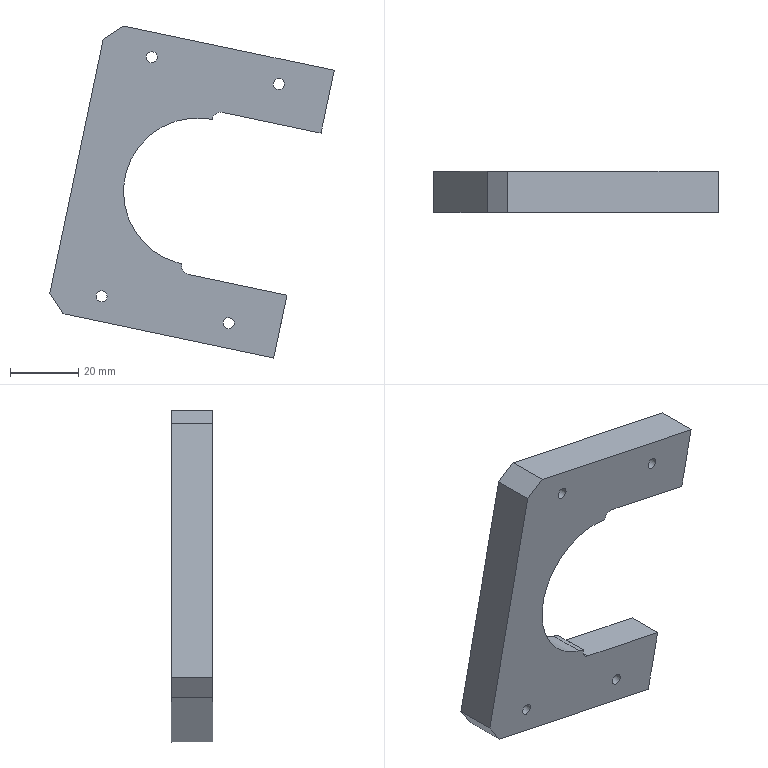Part | STEP file | BERCO_005 | 1 solid | 35 faces | box 83.204 x 12 x 97.117 mm | volume 41261 mm3 | plane 24 | cylinder 11 | commonest cylinder face diameters 3.242 x4 5 x4 42.992 x1 43 x1 52 x1